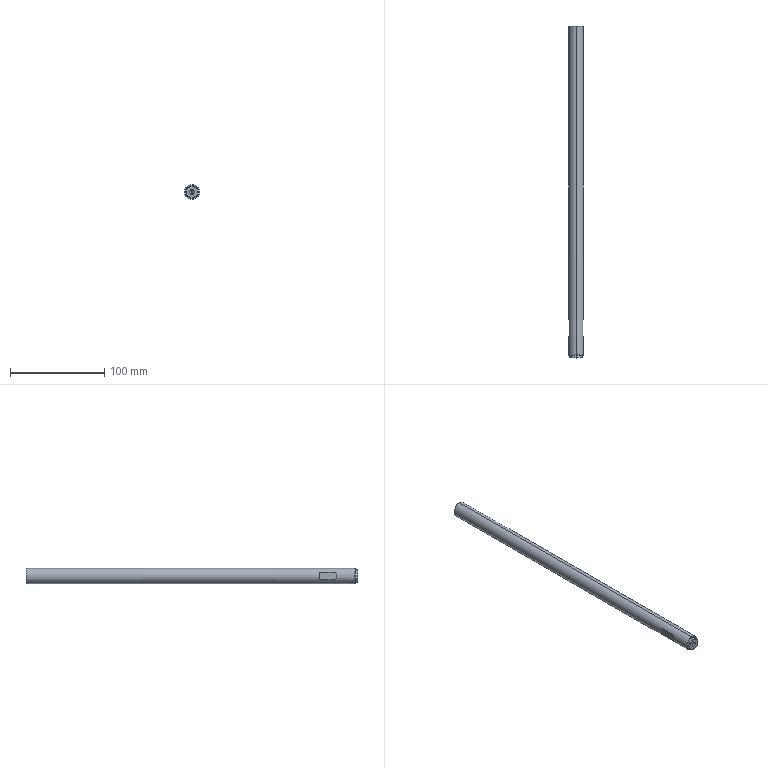Part | SolidWorks | features Chamfer 2, HoleWzd 2, ICE 2, Extrusion 1, MirrorPattern 1 | 1 solid | 27 faces | box 16 x 353 x 16 mm | volume 69897 mm3 | cone 10 | plane 9 | cylinder 8 | commonest cylinder face diameters 5 x4 13 x2 16 x2
STEP:
#1=CARTESIAN_POINT('',(0.,175.,7.5));
#2=VERTEX_POINT('',#1);
#3=CARTESIAN_POINT('',(0.,175.,-7.5));
#4=VERTEX_POINT('',#3);
#5=CARTESIAN_POINT('',(0.,175.,0.));
#6=DIRECTION('',(0.,1.,0.));
#7=DIRECTION('',(0.,0.,1.));
#8=AXIS2_PLACEMENT_3D('',#5,#6,#7);
#9=CIRCLE('',#8,7.5);
#10=EDGE_CURVE('',#2,#4,#9,.T.);
#11=ORIENTED_EDGE('',*,*,#10,.F.);
#12=CARTESIAN_POINT('',(0.,174.5,8.));
#13=VERTEX_POINT('',#12);
#14=CARTESIAN_POINT('',(0.,175.,7.5));
#15=DIRECTION('',(0.,-0.7071,0.7071));
#16=VECTOR('',#15,1000.);
#17=LINE('',#14,#16);
#18=EDGE_CURVE('',#2,#13,#17,.T.);
#19=ORIENTED_EDGE('',*,*,#18,.T.);
#20=CARTESIAN_POINT('',(0.,174.5,-8.));
#21=VERTEX_POINT('',#20);
#22=CARTESIAN_POINT('',(0.,174.5,0.));
#23=DIRECTION('',(0.,-1.,0.));
#24=DIRECTION('',(0.,0.,1.));
#25=AXIS2_PLACEMENT_3D('',#22,#23,#24);
#26=CIRCLE('',#25,8.);
#27=EDGE_CURVE('',#21,#13,#26,.T.);
#28=ORIENTED_EDGE('',*,*,#27,.F.);
#29=CARTESIAN_POINT('',(0.,175.,-7.5));
#30=DIRECTION('',(0.,-0.7071,-0.7071));
#31=VECTOR('',#30,1000.);
#32=LINE('',#29,#31);
#33=EDGE_CURVE('',#4,#21,#32,.T.);
#34=ORIENTED_EDGE('',*,*,#33,.F.);
#35=EDGE_LOOP('',(#11,#19,#28,#34));
#36=FACE_OUTER_BOUND('',#35,.T.);
#37=CARTESIAN_POINT('',(0.,175.,0.));
#38=DIRECTION('',(0.,-1.,0.));
#39=DIRECTION('',(0.,0.,-1.));
#40=AXIS2_PLACEMENT_3D('',#37,#38,#39);
#41=CONICAL_SURFACE('',#40,7.5,0.7854);
#42=ADVANCED_FACE('',(#36),#41,.T.);
#43=CARTESIAN_POINT('',(0.,-178.,-6.));
#44=VERTEX_POINT('',#43);
#45=CARTESIAN_POINT('',(0.,-178.,6.));
#46=VERTEX_POINT('',#45);
#47=CARTESIAN_POINT('',(0.,-178.,0.));
#48=DIRECTION('',(0.,-1.,0.));
#49=DIRECTION('',(0.,0.,-1.));
#50=AXIS2_PLACEMENT_3D('',#47,#48,#49);
#51=CIRCLE('',#50,6.);
#52=EDGE_CURVE('',#44,#46,#51,.T.);
#53=ORIENTED_EDGE('',*,*,#52,.F.);
#54=CARTESIAN_POINT('',(0.,-177.5,-6.5));
#55=VERTEX_POINT('',#54);
#56=CARTESIAN_POINT('',(0.,-178.,-6.));
#57=DIRECTION('',(0.,0.7071,-0.7071));
#58=VECTOR('',#57,1000.);
#59=LINE('',#56,#58);
#60=EDGE_CURVE('',#44,#55,#59,.T.);
#61=ORIENTED_EDGE('',*,*,#60,.T.);
#62=CARTESIAN_POINT('',(0.,-177.5,6.5));
#63=VERTEX_POINT('',#62);
#64=CARTESIAN_POINT('',(0.,-177.5,0.));
#65=DIRECTION('',(0.,1.,0.));
#66=DIRECTION('',(0.,0.,-1.));
#67=AXIS2_PLACEMENT_3D('',#64,#65,#66);
#68=CIRCLE('',#67,6.5);
#69=EDGE_CURVE('',#63,#55,#68,.T.);
#70=ORIENTED_EDGE('',*,*,#69,.F.);
#71=CARTESIAN_POINT('',(0.,-178.,6.));
#72=DIRECTION('',(0.,0.7071,0.7071));
#73=VECTOR('',#72,1000.);
#74=LINE('',#71,#73);
#75=EDGE_CURVE('',#46,#63,#74,.T.);
#76=ORIENTED_EDGE('',*,*,#75,.F.);
#77=EDGE_LOOP('',(#53,#61,#70,#76));
#78=FACE_OUTER_BOUND('',#77,.T.);
#79=CARTESIAN_POINT('',(0.,-178.,0.));
#80=DIRECTION('',(0.,1.,0.));
#81=DIRECTION('',(0.,0.,1.));
#82=AXIS2_PLACEMENT_3D('',#79,#80,#81);
#83=CONICAL_SURFACE('',#82,6.,0.7854);
#84=ADVANCED_FACE('',(#78),#83,.T.);
#85=CARTESIAN_POINT('',(0.,-175.,-7.5));
#86=VERTEX_POINT('',#85);
#87=CARTESIAN_POINT('',(0.,-175.,7.5));
#88=VERTEX_POINT('',#87);
#89=CARTESIAN_POINT('',(0.,-175.,0.));
#90=DIRECTION('',(0.,-1.,0.));
#91=DIRECTION('',(0.,0.,1.));
#92=AXIS2_PLACEMENT_3D('',#89,#90,#91);
#93=CIRCLE('',#92,7.5);
#94=EDGE_CURVE('',#86,#88,#93,.T.);
#95=ORIENTED_EDGE('',*,*,#94,.F.);
#96=CARTESIAN_POINT('',(0.,-174.5,-8.));
#97=VERTEX_POINT('',#96);
#98=CARTESIAN_POINT('',(0.,-174.5,-8.));
#99=DIRECTION('',(0.,0.7071,-0.7071));
#100=VECTOR('',#99,1000.);
#101=LINE('',#98,#100);
#102=EDGE_CURVE('',#86,#97,#101,.T.);
#103=ORIENTED_EDGE('',*,*,#102,.T.);
#104=CARTESIAN_POINT('',(0.,-174.5,8.));
#105=VERTEX_POINT('',#104);
#106=CARTESIAN_POINT('',(0.,-174.5,0.));
#107=DIRECTION('',(0.,1.,0.));
#108=DIRECTION('',(0.,0.,1.));
#109=AXIS2_PLACEMENT_3D('',#106,#107,#108);
#110=CIRCLE('',#109,8.);
#111=EDGE_CURVE('',#105,#97,#110,.T.);
#112=ORIENTED_EDGE('',*,*,#111,.F.);
#113=CARTESIAN_POINT('',(0.,-174.5,8.));
#114=DIRECTION('',(0.,0.7071,0.7071));
#115=VECTOR('',#114,1000.);
#116=LINE('',#113,#115);
#117=EDGE_CURVE('',#88,#105,#116,.T.);
#118=ORIENTED_EDGE('',*,*,#117,.F.);
#119=EDGE_LOOP('',(#95,#103,#112,#118));
#120=FACE_OUTER_BOUND('',#119,.T.);
#121=CARTESIAN_POINT('',(0.,-174.5,0.));
#122=DIRECTION('',(0.,1.,0.));
#123=DIRECTION('',(0.,0.,1.));
#124=AXIS2_PLACEMENT_3D('',#121,#122,#123);
#125=CONICAL_SURFACE('',#124,8.,0.7854);
#126=ADVANCED_FACE('',(#120),#125,.T.);
#127=ORIENTED_EDGE('',*,*,#69,.T.);
#128=CARTESIAN_POINT('',(0.,-175.,-6.5));
#129=VERTEX_POINT('',#128);
#130=CARTESIAN_POINT('',(0.,-178.,-6.5));
#131=DIRECTION('',(0.,1.,0.));
#132=VECTOR('',#131,1000.);
#133=LINE('',#130,#132);
#134=EDGE_CURVE('',#55,#129,#133,.T.);
#135=ORIENTED_EDGE('',*,*,#134,.T.);
#136=CARTESIAN_POINT('',(0.,-175.,6.5));
#137=VERTEX_POINT('',#136);
#138=CARTESIAN_POINT('',(0.,-175.,0.));
#139=DIRECTION('',(0.,-1.,0.));
#140=DIRECTION('',(0.,0.,-1.));
#141=AXIS2_PLACEMENT_3D('',#138,#139,#140);
#142=CIRCLE('',#141,6.5);
#143=EDGE_CURVE('',#129,#137,#142,.T.);
#144=ORIENTED_EDGE('',*,*,#143,.T.);
#145=CARTESIAN_POINT('',(0.,-178.,6.5));
#146=DIRECTION('',(0.,1.,0.));
#147=VECTOR('',#146,1000.);
#148=LINE('',#145,#147);
#149=EDGE_CURVE('',#63,#137,#148,.T.);
#150=ORIENTED_EDGE('',*,*,#149,.F.);
#151=EDGE_LOOP('',(#127,#135,#144,#150));
#152=FACE_OUTER_BOUND('',#151,.T.);
#153=CARTESIAN_POINT('',(0.,-178.,0.));
#154=DIRECTION('',(0.,1.,0.));
#155=DIRECTION('',(0.,0.,1.));
#156=AXIS2_PLACEMENT_3D('',#153,#154,#155);
#157=CYLINDRICAL_SURFACE('',#156,6.5);
#158=ADVANCED_FACE('',(#152),#157,.T.);
#159=CARTESIAN_POINT('',(0.,160.,-2.5));
#160=VERTEX_POINT('',#159);
#161=CARTESIAN_POINT('',(0.,160.,2.5));
#162=VERTEX_POINT('',#161);
#163=CARTESIAN_POINT('',(0.,160.,0.));
#164=DIRECTION('',(0.,1.,0.));
#165=DIRECTION('',(0.,0.,1.));
#166=AXIS2_PLACEMENT_3D('',#163,#164,#165);
#167=CIRCLE('',#166,2.5);
#168=EDGE_CURVE('',#160,#162,#167,.T.);
#169=ORIENTED_EDGE('',*,*,#168,.F.);
#170=CARTESIAN_POINT('',(0.,175.,-2.5));
#171=VERTEX_POINT('',#170);
#172=CARTESIAN_POINT('',(0.,175.,-2.5));
#173=DIRECTION('',(0.,1.,0.));
#174=VECTOR('',#173,1000.);
#175=LINE('',#172,#174);
#176=EDGE_CURVE('',#160,#171,#175,.T.);
#177=ORIENTED_EDGE('',*,*,#176,.T.);
#178=CARTESIAN_POINT('',(0.,175.,2.5));
#179=VERTEX_POINT('',#178);
#180=CARTESIAN_POINT('',(0.,175.,0.));
#181=DIRECTION('',(0.,1.,0.));
#182=DIRECTION('',(0.,0.,1.));
#183=AXIS2_PLACEMENT_3D('',#180,#181,#182);
#184=CIRCLE('',#183,2.5);
#185=EDGE_CURVE('',#171,#179,#184,.T.);
#186=ORIENTED_EDGE('',*,*,#185,.T.);
#187=CARTESIAN_POINT('',(0.,175.,2.5));
#188=DIRECTION('',(0.,1.,0.));
#189=VECTOR('',#188,1000.);
#190=LINE('',#187,#189);
#191=EDGE_CURVE('',#162,#179,#190,.T.);
#192=ORIENTED_EDGE('',*,*,#191,.F.);
#193=EDGE_LOOP('',(#169,#177,#186,#192));
#194=FACE_OUTER_BOUND('',#193,.T.);
#195=CARTESIAN_POINT('',(0.,175.,0.));
#196=DIRECTION('',(0.,1.,0.));
#197=DIRECTION('',(0.,0.,1.));
#198=AXIS2_PLACEMENT_3D('',#195,#196,#197);
#199=CYLINDRICAL_SURFACE('',#198,2.5);
#200=ADVANCED_FACE('',(#194),#199,.F.);
#201=CARTESIAN_POINT('',(0.,158.498,0.));
#202=VERTEX_POINT('',#201);
#203=CARTESIAN_POINT('',(0.,160.,2.5));
#204=DIRECTION('',(0.,0.515,0.8572));
#205=VECTOR('',#204,1000.);
#206=LINE('',#203,#205);
#207=EDGE_CURVE('',#202,#162,#206,.T.);
#208=ORIENTED_EDGE('',*,*,#207,.F.);
#209=CARTESIAN_POINT('',(0.,160.,-2.5));
#210=DIRECTION('',(0.,0.515,-0.8572));
#211=VECTOR('',#210,1000.);
#212=LINE('',#209,#211);
#213=EDGE_CURVE('',#202,#160,#212,.T.);
#214=ORIENTED_EDGE('',*,*,#213,.T.);
#215=ORIENTED_EDGE('',*,*,#168,.T.);
#216=EDGE_LOOP('',(#208,#214,#215));
#217=FACE_OUTER_BOUND('',#216,.T.);
#218=CARTESIAN_POINT('',(0.,160.,0.));
#219=DIRECTION('',(0.,1.,0.));
#220=DIRECTION('',(0.,0.,1.));
#221=AXIS2_PLACEMENT_3D('',#218,#219,#220);
#222=CONICAL_SURFACE('',#221,2.5,1.03);
#223=ADVANCED_FACE('',(#217),#222,.F.);
#224=CARTESIAN_POINT('',(7.,-137.,3.873));
#225=VERTEX_POINT('',#224);
#226=CARTESIAN_POINT('',(7.,-155.,3.873));
#227=VERTEX_POINT('',#226);
#228=CARTESIAN_POINT('',(7.,175.,3.873));
#229=DIRECTION('',(0.,-1.,0.));
#230=VECTOR('',#229,1000.);
#231=LINE('',#228,#230);
#232=EDGE_CURVE('',#225,#227,#231,.T.);
#233=ORIENTED_EDGE('',*,*,#232,.F.);
#234=CARTESIAN_POINT('',(7.,-137.,-3.873));
#235=VERTEX_POINT('',#234);
#236=CARTESIAN_POINT('',(0.,-137.,0.));
#237=DIRECTION('',(0.,-1.,0.));
#238=DIRECTION('',(0.,0.,-1.));
#239=AXIS2_PLACEMENT_3D('',#236,#237,#238);
#240=CIRCLE('',#239,8.);
#241=EDGE_CURVE('',#235,#225,#240,.T.);
#242=ORIENTED_EDGE('',*,*,#241,.F.);
#243=CARTESIAN_POINT('',(7.,-155.,-3.873));
#244=VERTEX_POINT('',#243);
#245=CARTESIAN_POINT('',(7.,175.,-3.873));
#246=DIRECTION('',(0.,1.,0.));
#247=VECTOR('',#246,1000.);
#248=LINE('',#245,#247);
#249=EDGE_CURVE('',#244,#235,#248,.T.);
#250=ORIENTED_EDGE('',*,*,#249,.F.);
#251=CARTESIAN_POINT('',(0.,-155.,0.));
#252=DIRECTION('',(0.,-1.,0.));
#253=DIRECTION('',(0.,0.,-1.));
#254=AXIS2_PLACEMENT_3D('',#251,#252,#253);
#255=CIRCLE('',#254,8.);
#256=EDGE_CURVE('',#244,#227,#255,.T.);
#257=ORIENTED_EDGE('',*,*,#256,.T.);
#258=EDGE_LOOP('',(#233,#242,#250,#257));
#259=FACE_BOUND('',#258,.T.);
#260=ORIENTED_EDGE('',*,*,#27,.T.);
#261=CARTESIAN_POINT('',(0.,175.,8.));
#262=DIRECTION('',(0.,-1.,0.));
#263=VECTOR('',#262,1000.);
#264=LINE('',#261,#263);
#265=EDGE_CURVE('',#13,#105,#264,.T.);
#266=ORIENTED_EDGE('',*,*,#265,.T.);
#267=ORIENTED_EDGE('',*,*,#111,.T.);
#268=CARTESIAN_POINT('',(0.,175.,-8.));
#269=DIRECTION('',(0.,-1.,0.));
#270=VECTOR('',#269,1000.);
#271=LINE('',#268,#270);
#272=EDGE_CURVE('',#21,#97,#271,.T.);
#273=ORIENTED_EDGE('',*,*,#272,.F.);
#274=EDGE_LOOP('',(#260,#266,#267,#273));
#275=FACE_OUTER_BOUND('',#274,.T.);
#276=CARTESIAN_POINT('',(0.,175.,0.));
#277=DIRECTION('',(0.,-1.,0.));
#278=DIRECTION('',(0.,0.,-1.));
#279=AXIS2_PLACEMENT_3D('',#276,#277,#278);
#280=CYLINDRICAL_SURFACE('',#279,8.);
#281=ADVANCED_FACE('',(#259,#275),#280,.T.);
#282=CARTESIAN_POINT('',(0.,-160.,2.5));
#283=VERTEX_POINT('',#282);
#284=CARTESIAN_POINT('',(0.,-160.,-2.5));
#285=VERTEX_POINT('',#284);
#286=CARTESIAN_POINT('',(0.,-160.,0.));
#287=DIRECTION('',(0.,-1.,0.));
#288=DIRECTION('',(0.,0.,-1.));
#289=AXIS2_PLACEMENT_3D('',#286,#287,#288);
#290=CIRCLE('',#289,2.5);
#291=EDGE_CURVE('',#283,#285,#290,.T.);
#292=ORIENTED_EDGE('',*,*,#291,.F.);
#293=CARTESIAN_POINT('',(0.,-178.,2.5));
#294=VERTEX_POINT('',#293);
#295=CARTESIAN_POINT('',(0.,-175.,2.5));
#296=DIRECTION('',(0.,-1.,0.));
#297=VECTOR('',#296,1000.);
#298=LINE('',#295,#297);
#299=EDGE_CURVE('',#283,#294,#298,.T.);
#300=ORIENTED_EDGE('',*,*,#299,.T.);
#301=CARTESIAN_POINT('',(0.,-178.,-2.5));
#302=VERTEX_POINT('',#301);
#303=CARTESIAN_POINT('',(0.,-178.,0.));
#304=DIRECTION('',(0.,-1.,0.));
#305=DIRECTION('',(0.,0.,-1.));
#306=AXIS2_PLACEMENT_3D('',#303,#304,#305);
#307=CIRCLE('',#306,2.5);
#308=EDGE_CURVE('',#294,#302,#307,.T.);
#309=ORIENTED_EDGE('',*,*,#308,.T.);
#310=CARTESIAN_POINT('',(0.,-175.,-2.5));
#311=DIRECTION('',(0.,-1.,0.));
#312=VECTOR('',#311,1000.);
#313=LINE('',#310,#312);
#314=EDGE_CURVE('',#285,#302,#313,.T.);
#315=ORIENTED_EDGE('',*,*,#314,.F.);
#316=EDGE_LOOP('',(#292,#300,#309,#315));
#317=FACE_OUTER_BOUND('',#316,.T.);
#318=CARTESIAN_POINT('',(0.,-175.,0.));
#319=DIRECTION('',(0.,-1.,0.));
#320=DIRECTION('',(0.,0.,-1.));
#321=AXIS2_PLACEMENT_3D('',#318,#319,#320);
#322=CYLINDRICAL_SURFACE('',#321,2.5);
#323=ADVANCED_FACE('',(#317),#322,.F.);
#324=CARTESIAN_POINT('',(0.,-158.498,0.));
#325=VERTEX_POINT('',#324);
#326=CARTESIAN_POINT('',(0.,-160.,-2.5));
#327=DIRECTION('',(0.,-0.515,-0.8572));
#328=VECTOR('',#327,1000.);
#329=LINE('',#326,#328);
#330=EDGE_CURVE('',#325,#285,#329,.T.);
#331=ORIENTED_EDGE('',*,*,#330,.F.);
#332=CARTESIAN_POINT('',(0.,-160.,2.5));
#333=DIRECTION('',(0.,-0.515,0.8572));
#334=VECTOR('',#333,1000.);
#335=LINE('',#332,#334);
#336=EDGE_CURVE('',#325,#283,#335,.T.);
#337=ORIENTED_EDGE('',*,*,#336,.T.);
#338=ORIENTED_EDGE('',*,*,#291,.T.);
#339=EDGE_LOOP('',(#331,#337,#338));
#340=FACE_OUTER_BOUND('',#339,.T.);
#341=CARTESIAN_POINT('',(0.,-160.,0.));
#342=DIRECTION('',(0.,-1.,0.));
#343=DIRECTION('',(0.,0.,-1.));
#344=AXIS2_PLACEMENT_3D('',#341,#342,#343);
#345=CONICAL_SURFACE('',#344,2.5,1.03);
#346=ADVANCED_FACE('',(#340),#345,.F.);
#347=ORIENTED_EDGE('',*,*,#336,.F.);
#348=ORIENTED_EDGE('',*,*,#330,.T.);
#349=CARTESIAN_POINT('',(0.,-160.,0.));
#350=DIRECTION('',(0.,-1.,0.));
#351=DIRECTION('',(0.,0.,-1.));
#352=AXIS2_PLACEMENT_3D('',#349,#350,#351);
#353=CIRCLE('',#352,2.5);
#354=EDGE_CURVE('',#285,#283,#353,.T.);
#355=ORIENTED_EDGE('',*,*,#354,.T.);
#356=EDGE_LOOP('',(#347,#348,#355));
#357=FACE_OUTER_BOUND('',#356,.T.);
#358=CARTESIAN_POINT('',(0.,-160.,0.));
#359=DIRECTION('',(0.,-1.,0.));
#360=DIRECTION('',(0.,0.,-1.));
#361=AXIS2_PLACEMENT_3D('',#358,#359,#360);
#362=CONICAL_SURFACE('',#361,2.5,1.03);
#363=ADVANCED_FACE('',(#357),#362,.F.);
#364=ORIENTED_EDGE('',*,*,#299,.F.);
#365=ORIENTED_EDGE('',*,*,#354,.F.);
#366=ORIENTED_EDGE('',*,*,#314,.T.);
#367=CARTESIAN_POINT('',(0.,-178.,0.));
#368=DIRECTION('',(0.,-1.,0.));
#369=DIRECTION('',(0.,0.,-1.));
#370=AXIS2_PLACEMENT_3D('',#367,#368,#369);
#371=CIRCLE('',#370,2.5);
#372=EDGE_CURVE('',#302,#294,#371,.T.);
#373=ORIENTED_EDGE('',*,*,#372,.T.);
#374=EDGE_LOOP('',(#364,#365,#366,#373));
#375=FACE_OUTER_BOUND('',#374,.T.);
#376=CARTESIAN_POINT('',(0.,-175.,0.));
#377=DIRECTION('',(0.,-1.,0.));
#378=DIRECTION('',(0.,0.,-1.));
#379=AXIS2_PLACEMENT_3D('',#376,#377,#378);
#380=CYLINDRICAL_SURFACE('',#379,2.5);
#381=ADVANCED_FACE('',(#375),#380,.F.);
#382=ORIENTED_EDGE('',*,*,#265,.F.);
#383=CARTESIAN_POINT('',(0.,174.5,0.));
#384=DIRECTION('',(0.,-1.,0.));
#385=DIRECTION('',(0.,0.,1.));
#386=AXIS2_PLACEMENT_3D('',#383,#384,#385);
#387=CIRCLE('',#386,8.);
#388=EDGE_CURVE('',#13,#21,#387,.T.);
#389=ORIENTED_EDGE('',*,*,#388,.T.);
#390=ORIENTED_EDGE('',*,*,#272,.T.);
#391=CARTESIAN_POINT('',(0.,-174.5,0.));
#392=DIRECTION('',(0.,1.,0.));
#393=DIRECTION('',(0.,0.,1.));
#394=AXIS2_PLACEMENT_3D('',#391,#392,#393);
#395=CIRCLE('',#394,8.);
#396=EDGE_CURVE('',#97,#105,#395,.T.);
#397=ORIENTED_EDGE('',*,*,#396,.T.);
#398=EDGE_LOOP('',(#382,#389,#390,#397));
#399=FACE_OUTER_BOUND('',#398,.T.);
#400=CARTESIAN_POINT('',(-7.,-137.,-3.873));
#401=VERTEX_POINT('',#400);
#402=CARTESIAN_POINT('',(-7.,-155.,-3.873));
#403=VERTEX_POINT('',#402);
#404=CARTESIAN_POINT('',(-7.,175.,-3.873));
#405=DIRECTION('',(0.,-1.,0.));
#406=VECTOR('',#405,1000.);
#407=LINE('',#404,#406);
#408=EDGE_CURVE('',#401,#403,#407,.T.);
#409=ORIENTED_EDGE('',*,*,#408,.F.);
#410=CARTESIAN_POINT('',(-7.,-137.,3.873));
#411=VERTEX_POINT('',#410);
#412=CARTESIAN_POINT('',(0.,-137.,0.));
#413=DIRECTION('',(0.,-1.,0.));
#414=DIRECTION('',(0.,0.,-1.));
#415=AXIS2_PLACEMENT_3D('',#412,#413,#414);
#416=CIRCLE('',#415,8.);
#417=EDGE_CURVE('',#411,#401,#416,.T.);
#418=ORIENTED_EDGE('',*,*,#417,.F.);
#419=CARTESIAN_POINT('',(-7.,-155.,3.873));
#420=VERTEX_POINT('',#419);
#421=CARTESIAN_POINT('',(-7.,175.,3.873));
#422=DIRECTION('',(0.,1.,0.));
#423=VECTOR('',#422,1000.);
#424=LINE('',#421,#423);
#425=EDGE_CURVE('',#420,#411,#424,.T.);
#426=ORIENTED_EDGE('',*,*,#425,.F.);
#427=CARTESIAN_POINT('',(0.,-155.,0.));
#428=DIRECTION('',(0.,-1.,0.));
#429=DIRECTION('',(0.,0.,-1.));
#430=AXIS2_PLACEMENT_3D('',#427,#428,#429);
#431=CIRCLE('',#430,8.);
#432=EDGE_CURVE('',#420,#403,#431,.T.);
#433=ORIENTED_EDGE('',*,*,#432,.T.);
#434=EDGE_LOOP('',(#409,#418,#426,#433));
#435=FACE_BOUND('',#434,.T.);
#436=CARTESIAN_POINT('',(0.,175.,0.));
#437=DIRECTION('',(0.,-1.,0.));
#438=DIRECTION('',(0.,0.,-1.));
#439=AXIS2_PLACEMENT_3D('',#436,#437,#438);
#440=CYLINDRICAL_SURFACE('',#439,8.);
#441=ADVANCED_FACE('',(#399,#435),#440,.T.);
#442=CARTESIAN_POINT('',(0.,175.,0.));
#443=DIRECTION('',(0.,1.,0.));
#444=DIRECTION('',(0.,0.,1.));
#445=AXIS2_PLACEMENT_3D('',#442,#443,#444);
#446=CIRCLE('',#445,7.5);
#447=EDGE_CURVE('',#4,#2,#446,.T.);
#448=ORIENTED_EDGE('',*,*,#447,.T.);
#449=ORIENTED_EDGE('',*,*,#10,.T.);
#450=EDGE_LOOP('',(#448,#449));
#451=FACE_OUTER_BOUND('',#450,.T.);
#452=CARTESIAN_POINT('',(0.,175.,0.));
#453=DIRECTION('',(0.,1.,0.));
#454=DIRECTION('',(0.,0.,1.));
#455=AXIS2_PLACEMENT_3D('',#452,#453,#454);
#456=CIRCLE('',#455,2.5);
#457=EDGE_CURVE('',#179,#171,#456,.T.);
#458=ORIENTED_EDGE('',*,*,#457,.F.);
#459=ORIENTED_EDGE('',*,*,#185,.F.);
#460=EDGE_LOOP('',(#458,#459));
#461=FACE_BOUND('',#460,.T.);
#462=CARTESIAN_POINT('',(0.,175.,0.));
#463=DIRECTION('',(0.,1.,0.));
#464=DIRECTION('',(0.,0.,1.));
#465=AXIS2_PLACEMENT_3D('',#462,#463,#464);
#466=PLANE('',#465);
#467=ADVANCED_FACE('',(#451,#461),#466,.T.);
#468=CARTESIAN_POINT('',(0.,-175.,0.));
#469=DIRECTION('',(0.,-1.,0.));
#470=DIRECTION('',(0.,0.,1.));
#471=AXIS2_PLACEMENT_3D('',#468,#469,#470);
#472=CIRCLE('',#471,7.5);
#473=EDGE_CURVE('',#88,#86,#472,.T.);
#474=ORIENTED_EDGE('',*,*,#473,.T.);
#475=ORIENTED_EDGE('',*,*,#94,.T.);
#476=EDGE_LOOP('',(#474,#475));
#477=FACE_OUTER_BOUND('',#476,.T.);
#478=CARTESIAN_POINT('',(0.,-175.,0.));
#479=DIRECTION('',(0.,-1.,0.));
#480=DIRECTION('',(0.,0.,-1.));
#481=AXIS2_PLACEMENT_3D('',#478,#479,#480);
#482=CIRCLE('',#481,6.5);
#483=EDGE_CURVE('',#137,#129,#482,.T.);
#484=ORIENTED_EDGE('',*,*,#483,.F.);
#485=ORIENTED_EDGE('',*,*,#143,.F.);
#486=EDGE_LOOP('',(#484,#485));
#487=FACE_BOUND('',#486,.T.);
#488=CARTESIAN_POINT('',(0.,-175.,0.));
#489=DIRECTION('',(0.,1.,0.));
#490=DIRECTION('',(0.,0.,1.));
#491=AXIS2_PLACEMENT_3D('',#488,#489,#490);
#492=PLANE('',#491);
#493=ADVANCED_FACE('',(#477,#487),#492,.F.);
#494=ORIENTED_EDGE('',*,*,#213,.F.);
#495=ORIENTED_EDGE('',*,*,#207,.T.);
#496=CARTESIAN_POINT('',(0.,160.,0.));
#497=DIRECTION('',(0.,1.,0.));
#498=DIRECTION('',(0.,0.,1.));
#499=AXIS2_PLACEMENT_3D('',#496,#497,#498);
#500=CIRCLE('',#499,2.5);
#501=EDGE_CURVE('',#162,#160,#500,.T.);
#502=ORIENTED_EDGE('',*,*,#501,.T.);
#503=EDGE_LOOP('',(#494,#495,#502));
#504=FACE_OUTER_BOUND('',#503,.T.);
#505=CARTESIAN_POINT('',(0.,160.,0.));
#506=DIRECTION('',(0.,1.,0.));
#507=DIRECTION('',(0.,0.,1.));
#508=AXIS2_PLACEMENT_3D('',#505,#506,#507);
#509=CONICAL_SURFACE('',#508,2.5,1.03);
#510=ADVANCED_FACE('',(#504),#509,.F.);
#511=ORIENTED_EDGE('',*,*,#176,.F.);
#512=ORIENTED_EDGE('',*,*,#501,.F.);
#513=ORIENTED_EDGE('',*,*,#191,.T.);
#514=ORIENTED_EDGE('',*,*,#457,.T.);
#515=EDGE_LOOP('',(#511,#512,#513,#514));
#516=FACE_OUTER_BOUND('',#515,.T.);
#517=CARTESIAN_POINT('',(0.,175.,0.));
#518=DIRECTION('',(0.,1.,0.));
#519=DIRECTION('',(0.,0.,1.));
#520=AXIS2_PLACEMENT_3D('',#517,#518,#519);
#521=CYLINDRICAL_SURFACE('',#520,2.5);
#522=ADVANCED_FACE('',(#516),#521,.F.);
#523=ORIENTED_EDGE('',*,*,#408,.T.);
#524=CARTESIAN_POINT('',(-7.,-155.,15.095));
#525=DIRECTION('',(0.,0.,-1.));
#526=VECTOR('',#525,1000.);
#527=LINE('',#524,#526);
#528=EDGE_CURVE('',#420,#403,#527,.T.);
#529=ORIENTED_EDGE('',*,*,#528,.F.);
#530=ORIENTED_EDGE('',*,*,#425,.T.);
#531=CARTESIAN_POINT('',(-7.,-137.,15.095));
#532=DIRECTION('',(0.,0.,-1.));
#533=VECTOR('',#532,1000.);
#534=LINE('',#531,#533);
#535=EDGE_CURVE('',#411,#401,#534,.T.);
#536=ORIENTED_EDGE('',*,*,#535,.T.);
#537=EDGE_LOOP('',(#523,#529,#530,#536));
#538=FACE_OUTER_BOUND('',#537,.T.);
#539=CARTESIAN_POINT('',(-7.,-137.,15.095));
#540=DIRECTION('',(-1.,0.,0.));
#541=DIRECTION('',(0.,0.,1.));
#542=AXIS2_PLACEMENT_3D('',#539,#540,#541);
#543=PLANE('',#542);
#544=ADVANCED_FACE('',(#538),#543,.T.);
#545=ORIENTED_EDGE('',*,*,#528,.T.);
#546=ORIENTED_EDGE('',*,*,#432,.F.);
#547=EDGE_LOOP('',(#545,#546));
#548=FACE_OUTER_BOUND('',#547,.T.);
#549=CARTESIAN_POINT('',(0.,-155.,0.));
#550=DIRECTION('',(0.,-1.,0.));
#551=DIRECTION('',(0.,0.,-1.));
#552=AXIS2_PLACEMENT_3D('',#549,#550,#551);
#553=PLANE('',#552);
#554=ADVANCED_FACE('',(#548),#553,.F.);
#555=ORIENTED_EDGE('',*,*,#417,.T.);
#556=ORIENTED_EDGE('',*,*,#535,.F.);
#557=EDGE_LOOP('',(#555,#556));
#558=FACE_OUTER_BOUND('',#557,.T.);
#559=CARTESIAN_POINT('',(0.,-137.,0.));
#560=DIRECTION('',(0.,-1.,0.));
#561=DIRECTION('',(0.,0.,-1.));
#562=AXIS2_PLACEMENT_3D('',#559,#560,#561);
#563=PLANE('',#562);
#564=ADVANCED_FACE('',(#558),#563,.T.);
#565=ORIENTED_EDGE('',*,*,#241,.T.);
#566=CARTESIAN_POINT('',(7.,-137.,15.095));
#567=DIRECTION('',(0.,0.,1.));
#568=VECTOR('',#567,1000.);
#569=LINE('',#566,#568);
#570=EDGE_CURVE('',#235,#225,#569,.T.);
#571=ORIENTED_EDGE('',*,*,#570,.F.);
#572=EDGE_LOOP('',(#565,#571));
#573=FACE_OUTER_BOUND('',#572,.T.);
#574=CARTESIAN_POINT('',(0.,-137.,0.));
#575=DIRECTION('',(0.,-1.,0.));
#576=DIRECTION('',(0.,0.,-1.));
#577=AXIS2_PLACEMENT_3D('',#574,#575,#576);
#578=PLANE('',#577);
#579=ADVANCED_FACE('',(#573),#578,.T.);
#580=CARTESIAN_POINT('',(7.,-155.,15.095));
#581=DIRECTION('',(0.,0.,1.));
#582=VECTOR('',#581,1000.);
#583=LINE('',#580,#582);
#584=EDGE_CURVE('',#244,#227,#583,.T.);
#585=ORIENTED_EDGE('',*,*,#584,.T.);
#586=ORIENTED_EDGE('',*,*,#256,.F.);
#587=EDGE_LOOP('',(#585,#586));
#588=FACE_OUTER_BOUND('',#587,.T.);
#589=CARTESIAN_POINT('',(0.,-155.,0.));
#590=DIRECTION('',(0.,-1.,0.));
#591=DIRECTION('',(0.,0.,-1.));
#592=AXIS2_PLACEMENT_3D('',#589,#590,#591);
#593=PLANE('',#592);
#594=ADVANCED_FACE('',(#588),#593,.F.);
#595=ORIENTED_EDGE('',*,*,#232,.T.);
#596=ORIENTED_EDGE('',*,*,#584,.F.);
#597=ORIENTED_EDGE('',*,*,#249,.T.);
#598=ORIENTED_EDGE('',*,*,#570,.T.);
#599=EDGE_LOOP('',(#595,#596,#597,#598));
#600=FACE_OUTER_BOUND('',#599,.T.);
#601=CARTESIAN_POINT('',(7.,-137.,15.095));
#602=DIRECTION('',(1.,0.,0.));
#603=DIRECTION('',(0.,0.,-1.));
#604=AXIS2_PLACEMENT_3D('',#601,#602,#603);
#605=PLANE('',#604);
#606=ADVANCED_FACE('',(#600),#605,.T.);
#607=CARTESIAN_POINT('',(0.,-178.,0.));
#608=DIRECTION('',(0.,-1.,0.));
#609=DIRECTION('',(0.,0.,-1.));
#610=AXIS2_PLACEMENT_3D('',#607,#608,#609);
#611=CIRCLE('',#610,6.);
#612=EDGE_CURVE('',#46,#44,#611,.T.);
#613=ORIENTED_EDGE('',*,*,#612,.T.);
#614=ORIENTED_EDGE('',*,*,#52,.T.);
#615=EDGE_LOOP('',(#613,#614));
#616=FACE_OUTER_BOUND('',#615,.T.);
#617=ORIENTED_EDGE('',*,*,#372,.F.);
#618=ORIENTED_EDGE('',*,*,#308,.F.);
#619=EDGE_LOOP('',(#617,#618));
#620=FACE_BOUND('',#619,.T.);
#621=CARTESIAN_POINT('',(0.,-178.,0.));
#622=DIRECTION('',(0.,-1.,0.));
#623=DIRECTION('',(0.,0.,-1.));
#624=AXIS2_PLACEMENT_3D('',#621,#622,#623);
#625=PLANE('',#624);
#626=ADVANCED_FACE('',(#616,#620),#625,.T.);
#627=ORIENTED_EDGE('',*,*,#134,.F.);
#628=CARTESIAN_POINT('',(0.,-177.5,0.));
#629=DIRECTION('',(0.,1.,0.));
#630=DIRECTION('',(0.,0.,-1.));
#631=AXIS2_PLACEMENT_3D('',#628,#629,#630);
#632=CIRCLE('',#631,6.5);
#633=EDGE_CURVE('',#55,#63,#632,.T.);
#634=ORIENTED_EDGE('',*,*,#633,.T.);
#635=ORIENTED_EDGE('',*,*,#149,.T.);
#636=ORIENTED_EDGE('',*,*,#483,.T.);
#637=EDGE_LOOP('',(#627,#634,#635,#636));
#638=FACE_OUTER_BOUND('',#637,.T.);
#639=CARTESIAN_POINT('',(0.,-178.,0.));
#640=DIRECTION('',(0.,1.,0.));
#641=DIRECTION('',(0.,0.,1.));
#642=AXIS2_PLACEMENT_3D('',#639,#640,#641);
#643=CYLINDRICAL_SURFACE('',#642,6.5);
#644=ADVANCED_FACE('',(#638),#643,.T.);
#645=ORIENTED_EDGE('',*,*,#102,.F.);
#646=ORIENTED_EDGE('',*,*,#473,.F.);
#647=ORIENTED_EDGE('',*,*,#117,.T.);
#648=ORIENTED_EDGE('',*,*,#396,.F.);
#649=EDGE_LOOP('',(#645,#646,#647,#648));
#650=FACE_OUTER_BOUND('',#649,.T.);
#651=CARTESIAN_POINT('',(0.,-174.5,0.));
#652=DIRECTION('',(0.,1.,0.));
#653=DIRECTION('',(0.,0.,1.));
#654=AXIS2_PLACEMENT_3D('',#651,#652,#653);
#655=CONICAL_SURFACE('',#654,8.,0.7854);
#656=ADVANCED_FACE('',(#650),#655,.T.);
#657=ORIENTED_EDGE('',*,*,#60,.F.);
#658=ORIENTED_EDGE('',*,*,#612,.F.);
#659=ORIENTED_EDGE('',*,*,#75,.T.);
#660=ORIENTED_EDGE('',*,*,#633,.F.);
#661=EDGE_LOOP('',(#657,#658,#659,#660));
#662=FACE_OUTER_BOUND('',#661,.T.);
#663=CARTESIAN_POINT('',(0.,-178.,0.));
#664=DIRECTION('',(0.,1.,0.));
#665=DIRECTION('',(0.,0.,1.));
#666=AXIS2_PLACEMENT_3D('',#663,#664,#665);
#667=CONICAL_SURFACE('',#666,6.,0.7854);
#668=ADVANCED_FACE('',(#662),#667,.T.);
#669=ORIENTED_EDGE('',*,*,#18,.F.);
#670=ORIENTED_EDGE('',*,*,#447,.F.);
#671=ORIENTED_EDGE('',*,*,#33,.T.);
#672=ORIENTED_EDGE('',*,*,#388,.F.);
#673=EDGE_LOOP('',(#669,#670,#671,#672));
#674=FACE_OUTER_BOUND('',#673,.T.);
#675=CARTESIAN_POINT('',(0.,175.,0.));
#676=DIRECTION('',(0.,-1.,0.));
#677=DIRECTION('',(0.,0.,-1.));
#678=AXIS2_PLACEMENT_3D('',#675,#676,#677);
#679=CONICAL_SURFACE('',#678,7.5,0.7854);
#680=ADVANCED_FACE('',(#674),#679,.T.);
#681=CLOSED_SHELL('',(#42,#84,#126,#158,#200,#223,#281,#323,#346,#363,#381,#441,#467,#493,#510,#522,#544,#554,#564,#579,#594,#606,#626,#644,#656,#668,#680));
#682=MANIFOLD_SOLID_BREP('',#681);
#683=CARTESIAN_POINT('',(0.,0.,0.));
#684=DIRECTION('',(0.,0.,1.));
#685=DIRECTION('',(1.,0.,0.));
#686=AXIS2_PLACEMENT_3D('',#683,#684,#685);
#687=(LENGTH_UNIT()NAMED_UNIT(*)SI_UNIT(.MILLI.,.METRE.));
#688=UNCERTAINTY_MEASURE_WITH_UNIT(LENGTH_MEASURE(0.00001),#687,'','');
#689=(NAMED_UNIT(*)PLANE_ANGLE_UNIT()SI_UNIT($,.RADIAN.));
#690=(NAMED_UNIT(*)SI_UNIT($,.STERADIAN.)SOLID_ANGLE_UNIT());
#691=(GEOMETRIC_REPRESENTATION_CONTEXT(3)GLOBAL_UNCERTAINTY_ASSIGNED_CONTEXT((#688))GLOBAL_UNIT_ASSIGNED_CONTEXT((#687,#689,#690))REPRESENTATION_CONTEXT('',''));
#692=ADVANCED_BREP_SHAPE_REPRESENTATION('',(#682,#686),#691);